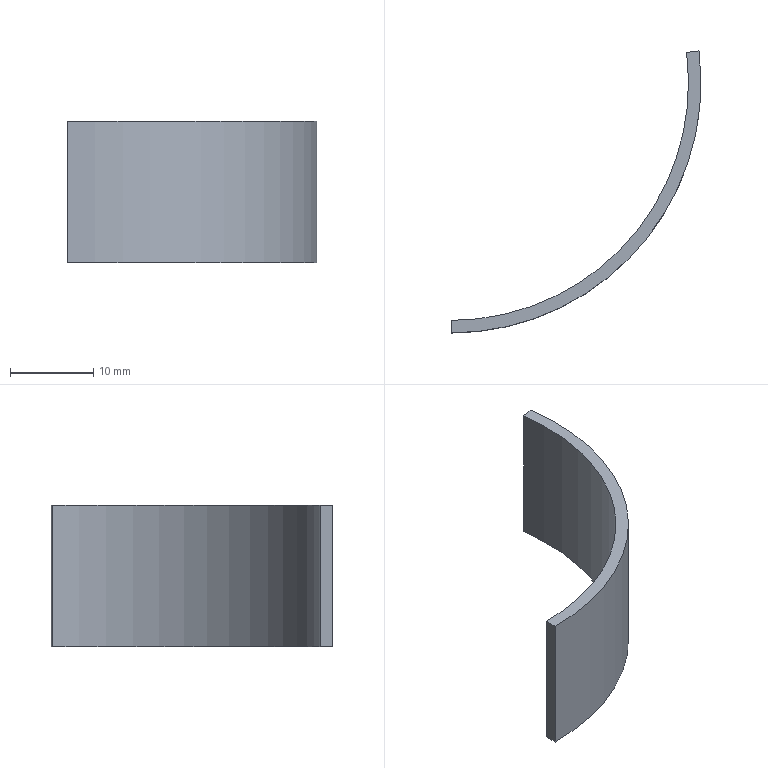Part | STEP file | FHD-021-012-C side door A-C | 1 solid | 6 faces | box 30 x 33.839 x 17 mm | volume 1267 mm3 | plane 4 | cylinder 2 | commonest cylinder face diameters 57 x1 60 x1
STEP:
#1=CARTESIAN_POINT('',(0.,0.,0.));
#2=DIRECTION('',(0.,0.,1.));
#3=DIRECTION('',(1.,0.,0.));
#4=AXIS2_PLACEMENT_3D('',#1,#2,#3);
#5=CARTESIAN_POINT('',(1916.338,859.802,17.));
#6=VERTEX_POINT('',#5);
#7=CARTESIAN_POINT('',(1886.585,825.963,17.));
#8=VERTEX_POINT('',#7);
#9=CARTESIAN_POINT('',(1886.585,855.963,17.));
#10=DIRECTION('',(0.,0.,-1.));
#11=DIRECTION('',(-1.,0.,0.));
#12=AXIS2_PLACEMENT_3D('',#9,#10,#11);
#13=CIRCLE('',#12,30.);
#14=CARTESIAN_POINT('',(1886.585,855.963,17.));
#15=DIRECTION('',(0.,0.,-1.));
#16=DIRECTION('',(-1.,0.,0.));
#17=AXIS2_PLACEMENT_3D('',#14,#15,#16);
#18=CYLINDRICAL_SURFACE('',#17,30.);
#19=CARTESIAN_POINT('',(0.,0.));
#20=DIRECTION('',(1.,0.));
#21=VECTOR('',#20,1.);
#22=LINE('',#19,#21);
#23=(GEOMETRIC_REPRESENTATION_CONTEXT(2)PARAMETRIC_REPRESENTATION_CONTEXT()REPRESENTATION_CONTEXT('',''));
#24=DEFINITIONAL_REPRESENTATION('',(#22),#23);
#25=PCURVE('',#18,#24);
#26=CARTESIAN_POINT('',(1886.585,855.963,17.));
#27=DIRECTION('',(0.,0.,1.));
#28=DIRECTION('',(1.,0.,0.));
#29=AXIS2_PLACEMENT_3D('',#26,#27,#28);
#30=PLANE('',#29);
#31=CARTESIAN_POINT('',(-30.,0.));
#32=CARTESIAN_POINT('',(-30.,51.962));
#33=CARTESIAN_POINT('',(15.,25.981));
#34=CARTESIAN_POINT('',(60.,0.));
#35=CARTESIAN_POINT('',(15.,-25.981));
#36=CARTESIAN_POINT('',(-30.,-51.962));
#37=CARTESIAN_POINT('',(-30.,0.));
#38=(BOUNDED_CURVE()B_SPLINE_CURVE(2,(#31,#32,#33,#34,#35,#36,#37),.UNSPECIFIED.,.T.,.F.)B_SPLINE_CURVE_WITH_KNOTS((1,2,2,2,2,1),(-2.094,0.,2.094,4.189,6.283,8.378),.UNSPECIFIED.)CURVE()GEOMETRIC_REPRESENTATION_ITEM()RATIONAL_B_SPLINE_CURVE((1.,0.5,1.,0.5,1.,0.5,1.))REPRESENTATION_ITEM(''));
#39=(GEOMETRIC_REPRESENTATION_CONTEXT(2)PARAMETRIC_REPRESENTATION_CONTEXT()REPRESENTATION_CONTEXT('',''));
#40=DEFINITIONAL_REPRESENTATION('',(#38),#39);
#41=PCURVE('',#30,#40);
#42=SURFACE_CURVE('',#13,(#25,#41),.PCURVE_S1.);
#43=EDGE_CURVE('',#6,#8,#42,.T.);
#44=ORIENTED_EDGE('',*,*,#43,.T.);
#45=CARTESIAN_POINT('',(1886.585,825.963,0.));
#46=VERTEX_POINT('',#45);
#47=CARTESIAN_POINT('',(1886.585,825.963,17.));
#48=DIRECTION('',(0.,0.,-1.));
#49=VECTOR('',#48,1.);
#50=LINE('',#47,#49);
#51=CARTESIAN_POINT('',(4.712,0.));
#52=DIRECTION('',(0.,1.));
#53=VECTOR('',#52,1.);
#54=LINE('',#51,#53);
#55=(GEOMETRIC_REPRESENTATION_CONTEXT(2)PARAMETRIC_REPRESENTATION_CONTEXT()REPRESENTATION_CONTEXT('',''));
#56=DEFINITIONAL_REPRESENTATION('',(#54),#55);
#57=PCURVE('',#18,#56);
#58=CARTESIAN_POINT('',(1886.585,825.963,17.));
#59=DIRECTION('',(-1.,0.,0.));
#60=DIRECTION('',(0.,0.,1.));
#61=AXIS2_PLACEMENT_3D('',#58,#59,#60);
#62=PLANE('',#61);
#63=CARTESIAN_POINT('',(0.,0.));
#64=DIRECTION('',(-1.,0.));
#65=VECTOR('',#64,1.);
#66=LINE('',#63,#65);
#67=(GEOMETRIC_REPRESENTATION_CONTEXT(2)PARAMETRIC_REPRESENTATION_CONTEXT()REPRESENTATION_CONTEXT('',''));
#68=DEFINITIONAL_REPRESENTATION('',(#66),#67);
#69=PCURVE('',#62,#68);
#70=SURFACE_CURVE('',#50,(#57,#69),.PCURVE_S1.);
#71=EDGE_CURVE('',#8,#46,#70,.T.);
#72=ORIENTED_EDGE('',*,*,#71,.T.);
#73=CARTESIAN_POINT('',(1916.338,859.802,0.));
#74=VERTEX_POINT('',#73);
#75=CARTESIAN_POINT('',(1886.585,855.963,0.));
#76=DIRECTION('',(0.,0.,1.));
#77=DIRECTION('',(-1.,0.,0.));
#78=AXIS2_PLACEMENT_3D('',#75,#76,#77);
#79=CIRCLE('',#78,30.);
#80=CARTESIAN_POINT('',(6.283,17.));
#81=DIRECTION('',(-1.,0.));
#82=VECTOR('',#81,1.);
#83=LINE('',#80,#82);
#84=(GEOMETRIC_REPRESENTATION_CONTEXT(2)PARAMETRIC_REPRESENTATION_CONTEXT()REPRESENTATION_CONTEXT('',''));
#85=DEFINITIONAL_REPRESENTATION('',(#83),#84);
#86=PCURVE('',#18,#85);
#87=CARTESIAN_POINT('',(1886.585,855.963,0.));
#88=DIRECTION('',(0.,0.,1.));
#89=DIRECTION('',(1.,0.,0.));
#90=AXIS2_PLACEMENT_3D('',#87,#88,#89);
#91=PLANE('',#90);
#92=CARTESIAN_POINT('',(0.,0.));
#93=DIRECTION('',(-1.,0.));
#94=AXIS2_PLACEMENT_2D('',#92,#93);
#95=CIRCLE('',#94,30.);
#96=(GEOMETRIC_REPRESENTATION_CONTEXT(2)PARAMETRIC_REPRESENTATION_CONTEXT()REPRESENTATION_CONTEXT('',''));
#97=DEFINITIONAL_REPRESENTATION('',(#95),#96);
#98=PCURVE('',#91,#97);
#99=SURFACE_CURVE('',#79,(#86,#98),.PCURVE_S1.);
#100=EDGE_CURVE('',#46,#74,#99,.T.);
#101=ORIENTED_EDGE('',*,*,#100,.T.);
#102=CARTESIAN_POINT('',(1916.338,859.802,17.));
#103=DIRECTION('',(0.,0.,1.));
#104=VECTOR('',#103,1.);
#105=LINE('',#102,#104);
#106=CARTESIAN_POINT('',(3.013,0.));
#107=DIRECTION('',(0.,-1.));
#108=VECTOR('',#107,1.);
#109=LINE('',#106,#108);
#110=(GEOMETRIC_REPRESENTATION_CONTEXT(2)PARAMETRIC_REPRESENTATION_CONTEXT()REPRESENTATION_CONTEXT('',''));
#111=DEFINITIONAL_REPRESENTATION('',(#109),#110);
#112=PCURVE('',#18,#111);
#113=CARTESIAN_POINT('',(1914.851,859.61,17.));
#114=DIRECTION('',(-0.128,0.9918,0.));
#115=DIRECTION('',(-0.9918,-0.128,0.));
#116=AXIS2_PLACEMENT_3D('',#113,#114,#115);
#117=PLANE('',#116);
#118=CARTESIAN_POINT('',(-1.5,0.));
#119=DIRECTION('',(0.,1.));
#120=VECTOR('',#119,1.);
#121=LINE('',#118,#120);
#122=(GEOMETRIC_REPRESENTATION_CONTEXT(2)PARAMETRIC_REPRESENTATION_CONTEXT()REPRESENTATION_CONTEXT('',''));
#123=DEFINITIONAL_REPRESENTATION('',(#121),#122);
#124=PCURVE('',#117,#123);
#125=SURFACE_CURVE('',#105,(#112,#124),.PCURVE_S1.);
#126=EDGE_CURVE('',#74,#6,#125,.T.);
#127=ORIENTED_EDGE('',*,*,#126,.T.);
#128=EDGE_LOOP('',(#44,#72,#101,#127));
#129=FACE_BOUND('',#128,.T.);
#130=ADVANCED_FACE('',(#129),#18,.T.);
#131=CARTESIAN_POINT('',(1886.585,827.463,17.));
#132=VERTEX_POINT('',#131);
#133=CARTESIAN_POINT('',(1886.585,825.963,17.));
#134=DIRECTION('',(0.,1.,0.));
#135=VECTOR('',#134,1.);
#136=LINE('',#133,#135);
#137=CARTESIAN_POINT('',(0.,0.));
#138=DIRECTION('',(0.,1.));
#139=VECTOR('',#138,1.);
#140=LINE('',#137,#139);
#141=(GEOMETRIC_REPRESENTATION_CONTEXT(2)PARAMETRIC_REPRESENTATION_CONTEXT()REPRESENTATION_CONTEXT('',''));
#142=DEFINITIONAL_REPRESENTATION('',(#140),#141);
#143=PCURVE('',#62,#142);
#144=CARTESIAN_POINT('',(0.,-30.));
#145=DIRECTION('',(0.,1.));
#146=VECTOR('',#145,1.);
#147=LINE('',#144,#146);
#148=(GEOMETRIC_REPRESENTATION_CONTEXT(2)PARAMETRIC_REPRESENTATION_CONTEXT()REPRESENTATION_CONTEXT('',''));
#149=DEFINITIONAL_REPRESENTATION('',(#147),#148);
#150=PCURVE('',#30,#149);
#151=SURFACE_CURVE('',#136,(#143,#150),.PCURVE_S1.);
#152=EDGE_CURVE('',#8,#132,#151,.T.);
#153=ORIENTED_EDGE('',*,*,#152,.T.);
#154=CARTESIAN_POINT('',(1886.585,827.463,0.));
#155=VERTEX_POINT('',#154);
#156=CARTESIAN_POINT('',(1886.585,827.463,17.));
#157=DIRECTION('',(0.,0.,-1.));
#158=VECTOR('',#157,1.);
#159=LINE('',#156,#158);
#160=CARTESIAN_POINT('',(0.,1.5));
#161=DIRECTION('',(-1.,0.));
#162=VECTOR('',#161,1.);
#163=LINE('',#160,#162);
#164=(GEOMETRIC_REPRESENTATION_CONTEXT(2)PARAMETRIC_REPRESENTATION_CONTEXT()REPRESENTATION_CONTEXT('',''));
#165=DEFINITIONAL_REPRESENTATION('',(#163),#164);
#166=PCURVE('',#62,#165);
#167=CARTESIAN_POINT('',(1886.585,855.963,17.));
#168=DIRECTION('',(0.,0.,-1.));
#169=DIRECTION('',(-1.,0.,0.));
#170=AXIS2_PLACEMENT_3D('',#167,#168,#169);
#171=CYLINDRICAL_SURFACE('',#170,28.5);
#172=CARTESIAN_POINT('',(4.712,0.));
#173=DIRECTION('',(0.,1.));
#174=VECTOR('',#173,1.);
#175=LINE('',#172,#174);
#176=(GEOMETRIC_REPRESENTATION_CONTEXT(2)PARAMETRIC_REPRESENTATION_CONTEXT()REPRESENTATION_CONTEXT('',''));
#177=DEFINITIONAL_REPRESENTATION('',(#175),#176);
#178=PCURVE('',#171,#177);
#179=SURFACE_CURVE('',#159,(#166,#178),.PCURVE_S1.);
#180=EDGE_CURVE('',#132,#155,#179,.T.);
#181=ORIENTED_EDGE('',*,*,#180,.T.);
#182=CARTESIAN_POINT('',(1886.585,825.963,0.));
#183=DIRECTION('',(0.,-1.,0.));
#184=VECTOR('',#183,1.);
#185=LINE('',#182,#184);
#186=CARTESIAN_POINT('',(-17.,0.));
#187=DIRECTION('',(0.,-1.));
#188=VECTOR('',#187,1.);
#189=LINE('',#186,#188);
#190=(GEOMETRIC_REPRESENTATION_CONTEXT(2)PARAMETRIC_REPRESENTATION_CONTEXT()REPRESENTATION_CONTEXT('',''));
#191=DEFINITIONAL_REPRESENTATION('',(#189),#190);
#192=PCURVE('',#62,#191);
#193=CARTESIAN_POINT('',(0.,-30.));
#194=DIRECTION('',(0.,-1.));
#195=VECTOR('',#194,1.);
#196=LINE('',#193,#195);
#197=(GEOMETRIC_REPRESENTATION_CONTEXT(2)PARAMETRIC_REPRESENTATION_CONTEXT()REPRESENTATION_CONTEXT('',''));
#198=DEFINITIONAL_REPRESENTATION('',(#196),#197);
#199=PCURVE('',#91,#198);
#200=SURFACE_CURVE('',#185,(#192,#199),.PCURVE_S1.);
#201=EDGE_CURVE('',#155,#46,#200,.T.);
#202=ORIENTED_EDGE('',*,*,#201,.T.);
#203=ORIENTED_EDGE('',*,*,#71,.F.);
#204=EDGE_LOOP('',(#153,#181,#202,#203));
#205=FACE_BOUND('',#204,.T.);
#206=ADVANCED_FACE('',(#205),#62,.T.);
#207=CARTESIAN_POINT('',(1914.851,859.61,17.));
#208=VERTEX_POINT('',#207);
#209=CARTESIAN_POINT('',(1886.585,855.963,17.));
#210=DIRECTION('',(0.,0.,-1.));
#211=DIRECTION('',(-1.,0.,0.));
#212=AXIS2_PLACEMENT_3D('',#209,#210,#211);
#213=CIRCLE('',#212,28.5);
#214=CARTESIAN_POINT('',(-28.5,0.));
#215=CARTESIAN_POINT('',(-28.5,49.363));
#216=CARTESIAN_POINT('',(14.25,24.682));
#217=CARTESIAN_POINT('',(57.,0.));
#218=CARTESIAN_POINT('',(14.25,-24.682));
#219=CARTESIAN_POINT('',(-28.5,-49.363));
#220=CARTESIAN_POINT('',(-28.5,0.));
#221=(BOUNDED_CURVE()B_SPLINE_CURVE(2,(#214,#215,#216,#217,#218,#219,#220),.UNSPECIFIED.,.T.,.F.)B_SPLINE_CURVE_WITH_KNOTS((1,2,2,2,2,1),(-2.094,0.,2.094,4.189,6.283,8.378),.UNSPECIFIED.)CURVE()GEOMETRIC_REPRESENTATION_ITEM()RATIONAL_B_SPLINE_CURVE((1.,0.5,1.,0.5,1.,0.5,1.))REPRESENTATION_ITEM(''));
#222=(GEOMETRIC_REPRESENTATION_CONTEXT(2)PARAMETRIC_REPRESENTATION_CONTEXT()REPRESENTATION_CONTEXT('',''));
#223=DEFINITIONAL_REPRESENTATION('',(#221),#222);
#224=PCURVE('',#30,#223);
#225=CARTESIAN_POINT('',(0.,0.));
#226=DIRECTION('',(1.,0.));
#227=VECTOR('',#226,1.);
#228=LINE('',#225,#227);
#229=(GEOMETRIC_REPRESENTATION_CONTEXT(2)PARAMETRIC_REPRESENTATION_CONTEXT()REPRESENTATION_CONTEXT('',''));
#230=DEFINITIONAL_REPRESENTATION('',(#228),#229);
#231=PCURVE('',#171,#230);
#232=SURFACE_CURVE('',#213,(#224,#231),.PCURVE_S1.);
#233=EDGE_CURVE('',#208,#132,#232,.T.);
#234=ORIENTED_EDGE('',*,*,#233,.T.);
#235=ORIENTED_EDGE('',*,*,#152,.F.);
#236=ORIENTED_EDGE('',*,*,#43,.F.);
#237=CARTESIAN_POINT('',(1916.338,859.802,17.));
#238=DIRECTION('',(-0.9918,-0.128,0.));
#239=VECTOR('',#238,1.);
#240=LINE('',#237,#239);
#241=CARTESIAN_POINT('',(29.753,3.839));
#242=DIRECTION('',(-0.9918,-0.128));
#243=VECTOR('',#242,1.);
#244=LINE('',#241,#243);
#245=(GEOMETRIC_REPRESENTATION_CONTEXT(2)PARAMETRIC_REPRESENTATION_CONTEXT()REPRESENTATION_CONTEXT('',''));
#246=DEFINITIONAL_REPRESENTATION('',(#244),#245);
#247=PCURVE('',#30,#246);
#248=CARTESIAN_POINT('',(-1.5,0.));
#249=DIRECTION('',(1.,0.));
#250=VECTOR('',#249,1.);
#251=LINE('',#248,#250);
#252=(GEOMETRIC_REPRESENTATION_CONTEXT(2)PARAMETRIC_REPRESENTATION_CONTEXT()REPRESENTATION_CONTEXT('',''));
#253=DEFINITIONAL_REPRESENTATION('',(#251),#252);
#254=PCURVE('',#117,#253);
#255=SURFACE_CURVE('',#240,(#247,#254),.PCURVE_S1.);
#256=EDGE_CURVE('',#6,#208,#255,.T.);
#257=ORIENTED_EDGE('',*,*,#256,.T.);
#258=EDGE_LOOP('',(#234,#235,#236,#257));
#259=FACE_BOUND('',#258,.T.);
#260=ADVANCED_FACE('',(#259),#30,.T.);
#261=ORIENTED_EDGE('',*,*,#256,.F.);
#262=ORIENTED_EDGE('',*,*,#126,.F.);
#263=CARTESIAN_POINT('',(1914.851,859.61,0.));
#264=VERTEX_POINT('',#263);
#265=CARTESIAN_POINT('',(1914.851,859.61,0.));
#266=DIRECTION('',(-0.9918,-0.128,0.));
#267=VECTOR('',#266,1.);
#268=LINE('',#265,#267);
#269=CARTESIAN_POINT('',(0.,-17.));
#270=DIRECTION('',(1.,0.));
#271=VECTOR('',#270,1.);
#272=LINE('',#269,#271);
#273=(GEOMETRIC_REPRESENTATION_CONTEXT(2)PARAMETRIC_REPRESENTATION_CONTEXT()REPRESENTATION_CONTEXT('',''));
#274=DEFINITIONAL_REPRESENTATION('',(#272),#273);
#275=PCURVE('',#117,#274);
#276=CARTESIAN_POINT('',(28.266,3.647));
#277=DIRECTION('',(-0.9918,-0.128));
#278=VECTOR('',#277,1.);
#279=LINE('',#276,#278);
#280=(GEOMETRIC_REPRESENTATION_CONTEXT(2)PARAMETRIC_REPRESENTATION_CONTEXT()REPRESENTATION_CONTEXT('',''));
#281=DEFINITIONAL_REPRESENTATION('',(#279),#280);
#282=PCURVE('',#91,#281);
#283=SURFACE_CURVE('',#268,(#275,#282),.PCURVE_S1.);
#284=EDGE_CURVE('',#74,#264,#283,.T.);
#285=ORIENTED_EDGE('',*,*,#284,.T.);
#286=CARTESIAN_POINT('',(1914.851,859.61,17.));
#287=DIRECTION('',(0.,0.,1.));
#288=VECTOR('',#287,1.);
#289=LINE('',#286,#288);
#290=CARTESIAN_POINT('',(0.,0.));
#291=DIRECTION('',(0.,1.));
#292=VECTOR('',#291,1.);
#293=LINE('',#290,#292);
#294=(GEOMETRIC_REPRESENTATION_CONTEXT(2)PARAMETRIC_REPRESENTATION_CONTEXT()REPRESENTATION_CONTEXT('',''));
#295=DEFINITIONAL_REPRESENTATION('',(#293),#294);
#296=PCURVE('',#117,#295);
#297=CARTESIAN_POINT('',(3.013,0.));
#298=DIRECTION('',(0.,-1.));
#299=VECTOR('',#298,1.);
#300=LINE('',#297,#299);
#301=(GEOMETRIC_REPRESENTATION_CONTEXT(2)PARAMETRIC_REPRESENTATION_CONTEXT()REPRESENTATION_CONTEXT('',''));
#302=DEFINITIONAL_REPRESENTATION('',(#300),#301);
#303=PCURVE('',#171,#302);
#304=SURFACE_CURVE('',#289,(#296,#303),.PCURVE_S1.);
#305=EDGE_CURVE('',#264,#208,#304,.T.);
#306=ORIENTED_EDGE('',*,*,#305,.T.);
#307=EDGE_LOOP('',(#261,#262,#285,#306));
#308=FACE_BOUND('',#307,.T.);
#309=ADVANCED_FACE('',(#308),#117,.T.);
#310=ORIENTED_EDGE('',*,*,#201,.F.);
#311=CARTESIAN_POINT('',(1886.585,855.963,0.));
#312=DIRECTION('',(0.,0.,-1.));
#313=DIRECTION('',(-1.,0.,0.));
#314=AXIS2_PLACEMENT_3D('',#311,#312,#313);
#315=CIRCLE('',#314,28.5);
#316=CARTESIAN_POINT('',(-28.5,0.));
#317=CARTESIAN_POINT('',(-28.5,49.363));
#318=CARTESIAN_POINT('',(14.25,24.682));
#319=CARTESIAN_POINT('',(57.,0.));
#320=CARTESIAN_POINT('',(14.25,-24.682));
#321=CARTESIAN_POINT('',(-28.5,-49.363));
#322=CARTESIAN_POINT('',(-28.5,0.));
#323=(BOUNDED_CURVE()B_SPLINE_CURVE(2,(#316,#317,#318,#319,#320,#321,#322),.UNSPECIFIED.,.T.,.F.)B_SPLINE_CURVE_WITH_KNOTS((1,2,2,2,2,1),(-2.094,0.,2.094,4.189,6.283,8.378),.UNSPECIFIED.)CURVE()GEOMETRIC_REPRESENTATION_ITEM()RATIONAL_B_SPLINE_CURVE((1.,0.5,1.,0.5,1.,0.5,1.))REPRESENTATION_ITEM(''));
#324=(GEOMETRIC_REPRESENTATION_CONTEXT(2)PARAMETRIC_REPRESENTATION_CONTEXT()REPRESENTATION_CONTEXT('',''));
#325=DEFINITIONAL_REPRESENTATION('',(#323),#324);
#326=PCURVE('',#91,#325);
#327=CARTESIAN_POINT('',(0.,17.));
#328=DIRECTION('',(1.,0.));
#329=VECTOR('',#328,1.);
#330=LINE('',#327,#329);
#331=(GEOMETRIC_REPRESENTATION_CONTEXT(2)PARAMETRIC_REPRESENTATION_CONTEXT()REPRESENTATION_CONTEXT('',''));
#332=DEFINITIONAL_REPRESENTATION('',(#330),#331);
#333=PCURVE('',#171,#332);
#334=SURFACE_CURVE('',#315,(#326,#333),.PCURVE_S1.);
#335=EDGE_CURVE('',#264,#155,#334,.T.);
#336=ORIENTED_EDGE('',*,*,#335,.F.);
#337=ORIENTED_EDGE('',*,*,#284,.F.);
#338=ORIENTED_EDGE('',*,*,#100,.F.);
#339=EDGE_LOOP('',(#310,#336,#337,#338));
#340=FACE_BOUND('',#339,.T.);
#341=ADVANCED_FACE('',(#340),#91,.F.);
#342=ORIENTED_EDGE('',*,*,#335,.F.);
#343=ORIENTED_EDGE('',*,*,#305,.T.);
#344=ORIENTED_EDGE('',*,*,#233,.T.);
#345=ORIENTED_EDGE('',*,*,#180,.T.);
#346=EDGE_LOOP('',(#342,#343,#344,#345));
#347=FACE_BOUND('',#346,.F.);
#348=ADVANCED_FACE('',(#347),#171,.F.);
#349=CLOSED_SHELL('',(#130,#206,#260,#309,#341,#348));
#350=MANIFOLD_SOLID_BREP('',#349);
#351=(LENGTH_UNIT()NAMED_UNIT(*)SI_UNIT(.MILLI.,.METRE.));
#352=UNCERTAINTY_MEASURE_WITH_UNIT(LENGTH_MEASURE(0.0000001),#351,'','');
#353=(NAMED_UNIT(*)PLANE_ANGLE_UNIT()SI_UNIT($,.RADIAN.));
#354=(NAMED_UNIT(*)SI_UNIT($,.STERADIAN.)SOLID_ANGLE_UNIT());
#355=(GEOMETRIC_REPRESENTATION_CONTEXT(3)GLOBAL_UNCERTAINTY_ASSIGNED_CONTEXT((#352))GLOBAL_UNIT_ASSIGNED_CONTEXT((#351,#353,#354))REPRESENTATION_CONTEXT('',''));
#356=ADVANCED_BREP_SHAPE_REPRESENTATION('',(#4,#350),#355);